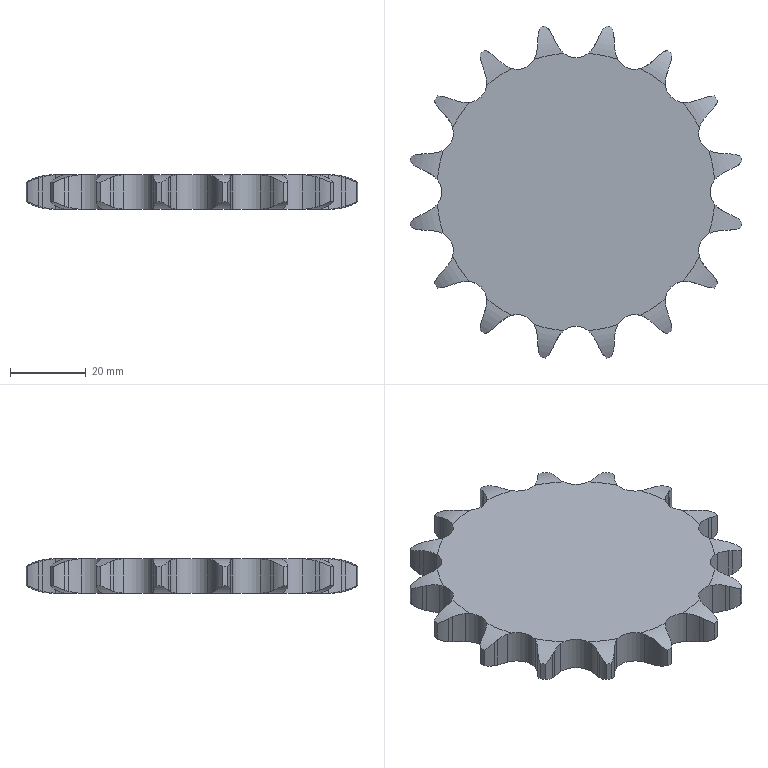Part | STEP file | Roller chain sprocket11 | 1 solid | 162 faces | box 87.888 x 87.888 x 9.168 mm | volume 42964 mm3 | cylinder 96 | plane 34 | torus 32 | commonest cylinder face diameters 16.939 x32 26.518 x32 10.262 x16 89.334 x16